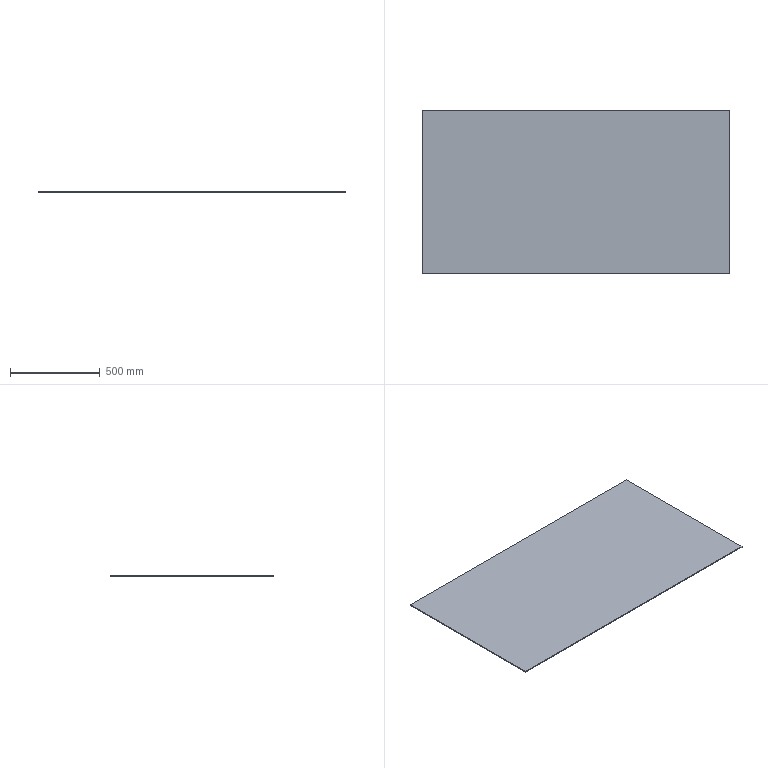Part | SolidWorks | features FlatPattern 1, SMBaseFlange 1, SheetMetal 1 | 1 solid | 6 faces | box 1704 x 910 x 5 mm | volume 7753200 mm3 | plane 6
STEP:
#1=CARTESIAN_POINT('',(0.,910.,0.));
#2=VERTEX_POINT('',#1);
#3=CARTESIAN_POINT('',(0.,0.,0.));
#4=VERTEX_POINT('',#3);
#5=CARTESIAN_POINT('',(0.,0.,0.));
#6=DIRECTION('',(0.,-1.,0.));
#7=VECTOR('',#6,1000.);
#8=LINE('',#5,#7);
#9=EDGE_CURVE('',#2,#4,#8,.T.);
#10=ORIENTED_EDGE('',*,*,#9,.F.);
#11=CARTESIAN_POINT('',(0.,910.,-5.));
#12=VERTEX_POINT('',#11);
#13=CARTESIAN_POINT('',(0.,910.,-5.));
#14=DIRECTION('',(0.,0.,1.));
#15=VECTOR('',#14,1000.);
#16=LINE('',#13,#15);
#17=EDGE_CURVE('',#12,#2,#16,.T.);
#18=ORIENTED_EDGE('',*,*,#17,.F.);
#19=CARTESIAN_POINT('',(0.,0.,-5.));
#20=VERTEX_POINT('',#19);
#21=CARTESIAN_POINT('',(0.,0.,-5.));
#22=DIRECTION('',(0.,-1.,0.));
#23=VECTOR('',#22,1000.);
#24=LINE('',#21,#23);
#25=EDGE_CURVE('',#12,#20,#24,.T.);
#26=ORIENTED_EDGE('',*,*,#25,.T.);
#27=CARTESIAN_POINT('',(0.,0.,-5.));
#28=DIRECTION('',(0.,0.,1.));
#29=VECTOR('',#28,1000.);
#30=LINE('',#27,#29);
#31=EDGE_CURVE('',#20,#4,#30,.T.);
#32=ORIENTED_EDGE('',*,*,#31,.T.);
#33=EDGE_LOOP('',(#10,#18,#26,#32));
#34=FACE_OUTER_BOUND('',#33,.T.);
#35=CARTESIAN_POINT('',(0.,0.,-5.));
#36=DIRECTION('',(-1.,0.,0.));
#37=DIRECTION('',(0.,0.,1.));
#38=AXIS2_PLACEMENT_3D('',#35,#36,#37);
#39=PLANE('',#38);
#40=ADVANCED_FACE('',(#34),#39,.T.);
#41=CARTESIAN_POINT('',(1704.,910.,0.));
#42=VERTEX_POINT('',#41);
#43=CARTESIAN_POINT('',(0.,910.,0.));
#44=DIRECTION('',(-1.,0.,0.));
#45=VECTOR('',#44,1000.);
#46=LINE('',#43,#45);
#47=EDGE_CURVE('',#42,#2,#46,.T.);
#48=ORIENTED_EDGE('',*,*,#47,.F.);
#49=CARTESIAN_POINT('',(1704.,910.,-5.));
#50=VERTEX_POINT('',#49);
#51=CARTESIAN_POINT('',(1704.,910.,-5.));
#52=DIRECTION('',(0.,0.,1.));
#53=VECTOR('',#52,1000.);
#54=LINE('',#51,#53);
#55=EDGE_CURVE('',#50,#42,#54,.T.);
#56=ORIENTED_EDGE('',*,*,#55,.F.);
#57=CARTESIAN_POINT('',(0.,910.,-5.));
#58=DIRECTION('',(-1.,0.,0.));
#59=VECTOR('',#58,1000.);
#60=LINE('',#57,#59);
#61=EDGE_CURVE('',#50,#12,#60,.T.);
#62=ORIENTED_EDGE('',*,*,#61,.T.);
#63=ORIENTED_EDGE('',*,*,#17,.T.);
#64=EDGE_LOOP('',(#48,#56,#62,#63));
#65=FACE_OUTER_BOUND('',#64,.T.);
#66=CARTESIAN_POINT('',(0.,910.,-5.));
#67=DIRECTION('',(0.,1.,0.));
#68=DIRECTION('',(0.,0.,1.));
#69=AXIS2_PLACEMENT_3D('',#66,#67,#68);
#70=PLANE('',#69);
#71=ADVANCED_FACE('',(#65),#70,.T.);
#72=CARTESIAN_POINT('',(1704.,0.,0.));
#73=VERTEX_POINT('',#72);
#74=CARTESIAN_POINT('',(1704.,0.,0.));
#75=DIRECTION('',(0.,1.,0.));
#76=VECTOR('',#75,1000.);
#77=LINE('',#74,#76);
#78=EDGE_CURVE('',#73,#42,#77,.T.);
#79=ORIENTED_EDGE('',*,*,#78,.F.);
#80=CARTESIAN_POINT('',(1704.,0.,-5.));
#81=VERTEX_POINT('',#80);
#82=CARTESIAN_POINT('',(1704.,0.,-5.));
#83=DIRECTION('',(0.,0.,1.));
#84=VECTOR('',#83,1000.);
#85=LINE('',#82,#84);
#86=EDGE_CURVE('',#81,#73,#85,.T.);
#87=ORIENTED_EDGE('',*,*,#86,.F.);
#88=CARTESIAN_POINT('',(1704.,0.,-5.));
#89=DIRECTION('',(0.,1.,0.));
#90=VECTOR('',#89,1000.);
#91=LINE('',#88,#90);
#92=EDGE_CURVE('',#81,#50,#91,.T.);
#93=ORIENTED_EDGE('',*,*,#92,.T.);
#94=ORIENTED_EDGE('',*,*,#55,.T.);
#95=EDGE_LOOP('',(#79,#87,#93,#94));
#96=FACE_OUTER_BOUND('',#95,.T.);
#97=CARTESIAN_POINT('',(1704.,0.,-5.));
#98=DIRECTION('',(1.,0.,0.));
#99=DIRECTION('',(0.,0.,-1.));
#100=AXIS2_PLACEMENT_3D('',#97,#98,#99);
#101=PLANE('',#100);
#102=ADVANCED_FACE('',(#96),#101,.T.);
#103=CARTESIAN_POINT('',(0.,0.,0.));
#104=DIRECTION('',(1.,0.,0.));
#105=VECTOR('',#104,1000.);
#106=LINE('',#103,#105);
#107=EDGE_CURVE('',#4,#73,#106,.T.);
#108=ORIENTED_EDGE('',*,*,#107,.F.);
#109=ORIENTED_EDGE('',*,*,#31,.F.);
#110=CARTESIAN_POINT('',(0.,0.,-5.));
#111=DIRECTION('',(1.,0.,0.));
#112=VECTOR('',#111,1000.);
#113=LINE('',#110,#112);
#114=EDGE_CURVE('',#20,#81,#113,.T.);
#115=ORIENTED_EDGE('',*,*,#114,.T.);
#116=ORIENTED_EDGE('',*,*,#86,.T.);
#117=EDGE_LOOP('',(#108,#109,#115,#116));
#118=FACE_OUTER_BOUND('',#117,.T.);
#119=CARTESIAN_POINT('',(0.,0.,-5.));
#120=DIRECTION('',(0.,-1.,0.));
#121=DIRECTION('',(0.,0.,-1.));
#122=AXIS2_PLACEMENT_3D('',#119,#120,#121);
#123=PLANE('',#122);
#124=ADVANCED_FACE('',(#118),#123,.T.);
#125=ORIENTED_EDGE('',*,*,#25,.F.);
#126=ORIENTED_EDGE('',*,*,#61,.F.);
#127=ORIENTED_EDGE('',*,*,#92,.F.);
#128=ORIENTED_EDGE('',*,*,#114,.F.);
#129=EDGE_LOOP('',(#125,#126,#127,#128));
#130=FACE_OUTER_BOUND('',#129,.T.);
#131=CARTESIAN_POINT('',(0.,0.,-5.));
#132=DIRECTION('',(0.,0.,-1.));
#133=DIRECTION('',(-1.,0.,0.));
#134=AXIS2_PLACEMENT_3D('',#131,#132,#133);
#135=PLANE('',#134);
#136=ADVANCED_FACE('',(#130),#135,.T.);
#137=ORIENTED_EDGE('',*,*,#9,.T.);
#138=ORIENTED_EDGE('',*,*,#107,.T.);
#139=ORIENTED_EDGE('',*,*,#78,.T.);
#140=ORIENTED_EDGE('',*,*,#47,.T.);
#141=EDGE_LOOP('',(#137,#138,#139,#140));
#142=FACE_OUTER_BOUND('',#141,.T.);
#143=CARTESIAN_POINT('',(0.,0.,0.));
#144=DIRECTION('',(0.,0.,-1.));
#145=DIRECTION('',(-1.,0.,0.));
#146=AXIS2_PLACEMENT_3D('',#143,#144,#145);
#147=PLANE('',#146);
#148=ADVANCED_FACE('',(#142),#147,.F.);
#149=CLOSED_SHELL('',(#40,#71,#102,#124,#136,#148));
#150=MANIFOLD_SOLID_BREP('',#149);
#151=CARTESIAN_POINT('',(0.,0.,0.));
#152=DIRECTION('',(0.,0.,1.));
#153=DIRECTION('',(1.,0.,0.));
#154=AXIS2_PLACEMENT_3D('',#151,#152,#153);
#155=(LENGTH_UNIT()NAMED_UNIT(*)SI_UNIT(.MILLI.,.METRE.));
#156=UNCERTAINTY_MEASURE_WITH_UNIT(LENGTH_MEASURE(0.00001),#155,'','');
#157=(NAMED_UNIT(*)PLANE_ANGLE_UNIT()SI_UNIT($,.RADIAN.));
#158=(NAMED_UNIT(*)SI_UNIT($,.STERADIAN.)SOLID_ANGLE_UNIT());
#159=(GEOMETRIC_REPRESENTATION_CONTEXT(3)GLOBAL_UNCERTAINTY_ASSIGNED_CONTEXT((#156))GLOBAL_UNIT_ASSIGNED_CONTEXT((#155,#157,#158))REPRESENTATION_CONTEXT('',''));
#160=ADVANCED_BREP_SHAPE_REPRESENTATION('',(#150,#154),#159);